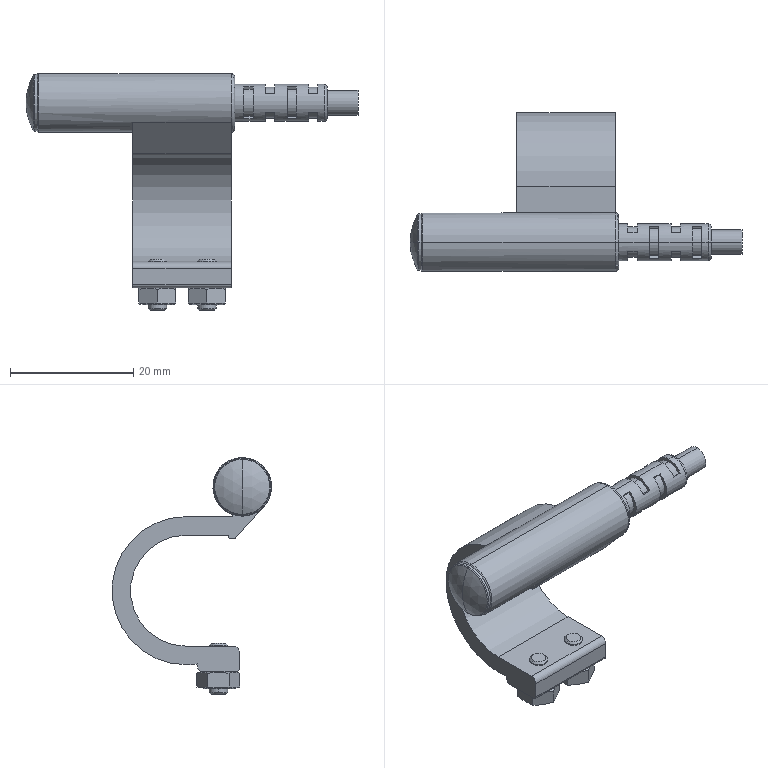Part | STEP file | CS1_B4 | 1 solid | 141 faces | box 53.8 x 25.85 x 38.4 mm | volume 5585 mm3 | plane 80 | cylinder 35 | cone 16 | torus 8 | sphere 2 | commonest cylinder face diameters 5 x10 3 x8 1 x2 2 x2 4 x2 6 x2